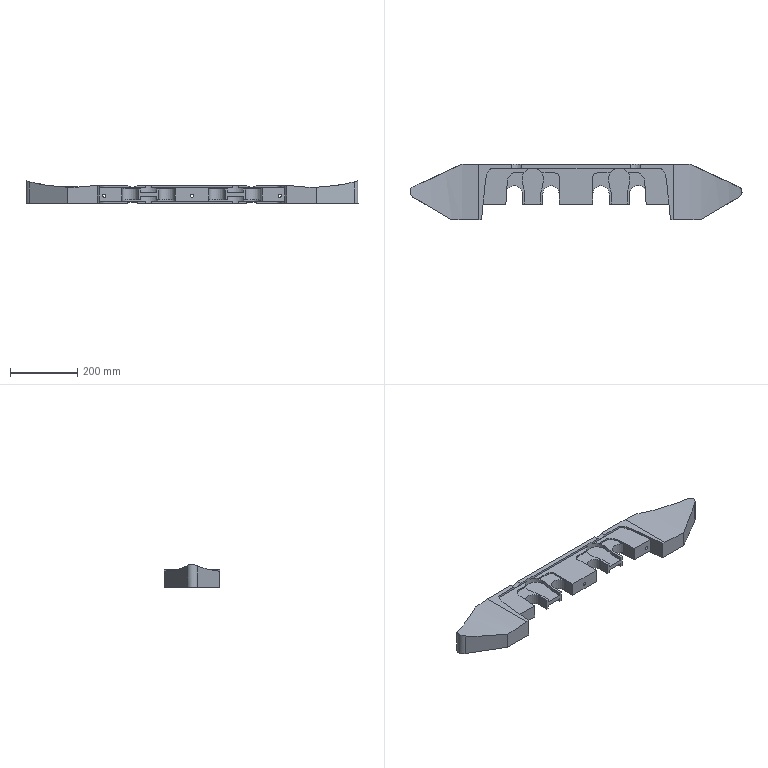Part | SolidWorks | features MirrorPattern 11, ICE 9, 3DProfileFeature 4, Extrusion 1 | 1 solid | 138 faces | box 984.004 x 165 x 67.16 mm | volume 4451171 mm3 | plane 86 | cylinder 30 | spline 22 | commonest cylinder face diameters 10 x6 25 x6 33 x6 64 x4 33.92 x2 47.646 x2